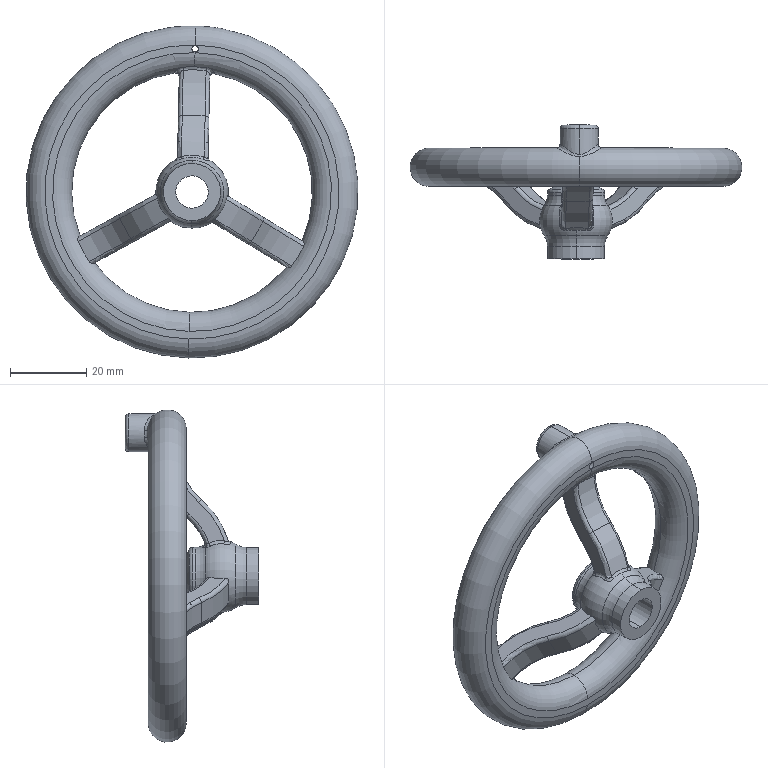Part | STEP file | Input 49 | 1 solid | 106 faces | box 87 x 35.001 x 87 mm | volume 30093 mm3 | torus 40 | cylinder 24 | spline 23 | plane 11 | cone 4 | other 2 | sphere 2 | commonest cylinder face diameters 34 x6 46 x6 15 x4 5 x2 6 x2 8.5 x2